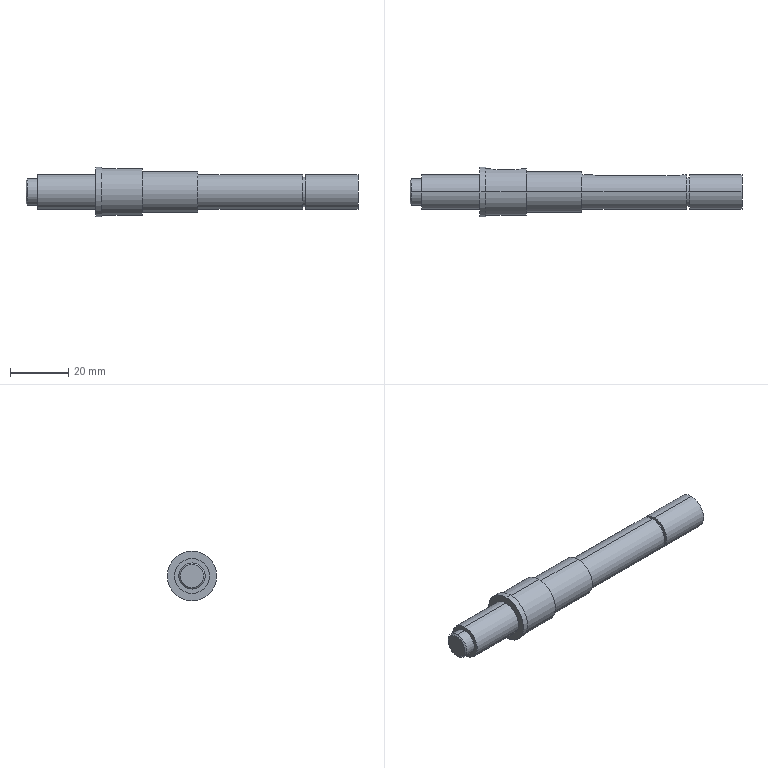Part | SolidWorks | features ICE 2, Revolution 1 | 1 solid | 39 faces | box 114 x 17 x 17 mm | volume 14497 mm3 | cylinder 22 | plane 15 | cone 2 | commonest cylinder face diameters 12 x6 4 x3 5 x3 9 x2 10 x2 14 x2
STEP:
#1=CARTESIAN_POINT('',(-42.725,5.2,0.));
#2=VERTEX_POINT('',#1);
#3=CARTESIAN_POINT('',(-40.225,5.2,2.5));
#4=VERTEX_POINT('',#3);
#5=CARTESIAN_POINT('',(-40.225,5.2,0.));
#6=DIRECTION('',(0.,1.,0.));
#7=DIRECTION('',(-1.,0.,0.));
#8=AXIS2_PLACEMENT_3D('',#5,#6,#7);
#9=CIRCLE('',#8,2.5);
#10=EDGE_CURVE('',#2,#4,#9,.T.);
#11=ORIENTED_EDGE('',*,*,#10,.F.);
#12=CARTESIAN_POINT('',(-42.725,8.,0.));
#13=VERTEX_POINT('',#12);
#14=CARTESIAN_POINT('',(-42.725,5.2,0.));
#15=DIRECTION('',(0.,1.,0.));
#16=VECTOR('',#15,1000.);
#17=LINE('',#14,#16);
#18=EDGE_CURVE('',#2,#13,#17,.T.);
#19=ORIENTED_EDGE('',*,*,#18,.T.);
#20=CARTESIAN_POINT('',(-40.225,7.599,2.5));
#21=VERTEX_POINT('',#20);
#22=CARTESIAN_POINT('',(-40.225,7.599,2.5));
#23=CARTESIAN_POINT('',(-40.392,7.599,2.5));
#24=CARTESIAN_POINT('',(-40.555,7.605,2.484));
#25=CARTESIAN_POINT('',(-40.876,7.625,2.419));
#26=CARTESIAN_POINT('',(-41.035,7.641,2.371));
#27=CARTESIAN_POINT('',(-41.338,7.679,2.245));
#28=CARTESIAN_POINT('',(-41.481,7.701,2.168));
#29=CARTESIAN_POINT('',(-41.752,7.75,1.986));
#30=CARTESIAN_POINT('',(-41.879,7.776,1.882));
#31=CARTESIAN_POINT('',(-42.223,7.854,1.538));
#32=CARTESIAN_POINT('',(-42.409,7.906,1.26));
#33=CARTESIAN_POINT('',(-42.596,7.96,0.8095));
#34=CARTESIAN_POINT('',(-42.645,7.975,0.6507));
#35=CARTESIAN_POINT('',(-42.709,7.995,0.3273));
#36=CARTESIAN_POINT('',(-42.725,8.,0.1643));
#37=CARTESIAN_POINT('',(-42.725,8.,0.));
#38=B_SPLINE_CURVE_WITH_KNOTS('',3,(#22,#23,#24,#25,#26,#27,#28,#29,#30,#31,#32,#33,#34,#35,#36,#37),.UNSPECIFIED.,.F.,.F.,(4,2,2,2,2,2,2,4),(0.,0.0004917,0.0009835,0.001475,0.001967,0.00295,0.003442,0.003934),.UNSPECIFIED.);
#39=EDGE_CURVE('',#21,#13,#38,.T.);
#40=ORIENTED_EDGE('',*,*,#39,.F.);
#41=CARTESIAN_POINT('',(-40.225,5.2,2.5));
#42=DIRECTION('',(0.,1.,0.));
#43=VECTOR('',#42,1000.);
#44=LINE('',#41,#43);
#45=EDGE_CURVE('',#4,#21,#44,.T.);
#46=ORIENTED_EDGE('',*,*,#45,.F.);
#47=EDGE_LOOP('',(#11,#19,#40,#46));
#48=FACE_OUTER_BOUND('',#47,.T.);
#49=CARTESIAN_POINT('',(-40.225,5.2,0.));
#50=DIRECTION('',(0.,1.,0.));
#51=DIRECTION('',(-1.,0.,0.));
#52=AXIS2_PLACEMENT_3D('',#49,#50,#51);
#53=CYLINDRICAL_SURFACE('',#52,2.5);
#54=ADVANCED_FACE('',(#48),#53,.F.);
#55=CARTESIAN_POINT('',(-8.054,3.8,0.));
#56=VERTEX_POINT('',#55);
#57=CARTESIAN_POINT('',(-6.054,3.8,2.));
#58=VERTEX_POINT('',#57);
#59=CARTESIAN_POINT('',(-6.054,3.8,0.));
#60=DIRECTION('',(0.,1.,0.));
#61=DIRECTION('',(-1.,0.,0.));
#62=AXIS2_PLACEMENT_3D('',#59,#60,#61);
#63=CIRCLE('',#62,2.);
#64=EDGE_CURVE('',#56,#58,#63,.T.);
#65=ORIENTED_EDGE('',*,*,#64,.F.);
#66=CARTESIAN_POINT('',(-8.054,6.,0.));
#67=VERTEX_POINT('',#66);
#68=CARTESIAN_POINT('',(-8.054,3.8,0.));
#69=DIRECTION('',(0.,1.,0.));
#70=VECTOR('',#69,1000.);
#71=LINE('',#68,#70);
#72=EDGE_CURVE('',#56,#67,#71,.T.);
#73=ORIENTED_EDGE('',*,*,#72,.T.);
#74=CARTESIAN_POINT('',(-6.054,5.657,2.));
#75=VERTEX_POINT('',#74);
#76=CARTESIAN_POINT('',(-6.054,5.657,2.));
#77=CARTESIAN_POINT('',(-6.187,5.657,2.));
#78=CARTESIAN_POINT('',(-6.318,5.662,1.987));
#79=CARTESIAN_POINT('',(-6.575,5.679,1.935));
#80=CARTESIAN_POINT('',(-6.702,5.693,1.896));
#81=CARTESIAN_POINT('',(-6.944,5.725,1.796));
#82=CARTESIAN_POINT('',(-7.059,5.744,1.734));
#83=CARTESIAN_POINT('',(-7.275,5.786,1.589));
#84=CARTESIAN_POINT('',(-7.377,5.809,1.505));
#85=CARTESIAN_POINT('',(-7.652,5.876,1.23));
#86=CARTESIAN_POINT('',(-7.8,5.92,1.009));
#87=CARTESIAN_POINT('',(-7.95,5.966,0.648));
#88=CARTESIAN_POINT('',(-7.989,5.979,0.5209));
#89=CARTESIAN_POINT('',(-8.041,5.996,0.2621));
#90=CARTESIAN_POINT('',(-8.054,6.,0.1316));
#91=CARTESIAN_POINT('',(-8.054,6.,0.));
#92=B_SPLINE_CURVE_WITH_KNOTS('',3,(#76,#77,#78,#79,#80,#81,#82,#83,#84,#85,#86,#87,#88,#89,#90,#91),.UNSPECIFIED.,.F.,.F.,(4,2,2,2,2,2,2,4),(0.,0.0003937,0.0007875,0.001181,0.001575,0.002362,0.002756,0.00315),.UNSPECIFIED.);
#93=EDGE_CURVE('',#75,#67,#92,.T.);
#94=ORIENTED_EDGE('',*,*,#93,.F.);
#95=CARTESIAN_POINT('',(-6.054,3.8,2.));
#96=DIRECTION('',(0.,1.,0.));
#97=VECTOR('',#96,1000.);
#98=LINE('',#95,#97);
#99=EDGE_CURVE('',#58,#75,#98,.T.);
#100=ORIENTED_EDGE('',*,*,#99,.F.);
#101=EDGE_LOOP('',(#65,#73,#94,#100));
#102=FACE_OUTER_BOUND('',#101,.T.);
#103=CARTESIAN_POINT('',(-6.054,3.8,0.));
#104=DIRECTION('',(0.,1.,0.));
#105=DIRECTION('',(-1.,0.,0.));
#106=AXIS2_PLACEMENT_3D('',#103,#104,#105);
#107=CYLINDRICAL_SURFACE('',#106,2.);
#108=ADVANCED_FACE('',(#102),#107,.F.);
#109=CARTESIAN_POINT('',(43.896,0.,6.));
#110=VERTEX_POINT('',#109);
#111=CARTESIAN_POINT('',(43.896,0.,-6.));
#112=VERTEX_POINT('',#111);
#113=CARTESIAN_POINT('',(43.896,0.,0.));
#114=DIRECTION('',(-1.,0.,0.));
#115=DIRECTION('',(0.,0.,1.));
#116=AXIS2_PLACEMENT_3D('',#113,#114,#115);
#117=CIRCLE('',#116,6.);
#118=EDGE_CURVE('',#110,#112,#117,.T.);
#119=ORIENTED_EDGE('',*,*,#118,.T.);
#120=CARTESIAN_POINT('',(25.896,0.,-6.));
#121=VERTEX_POINT('',#120);
#122=CARTESIAN_POINT('',(-70.104,0.,-6.));
#123=DIRECTION('',(-1.,0.,0.));
#124=VECTOR('',#123,1000.);
#125=LINE('',#122,#124);
#126=EDGE_CURVE('',#112,#121,#125,.T.);
#127=ORIENTED_EDGE('',*,*,#126,.T.);
#128=CARTESIAN_POINT('',(25.896,0.,6.));
#129=VERTEX_POINT('',#128);
#130=CARTESIAN_POINT('',(25.896,0.,0.));
#131=DIRECTION('',(-1.,0.,0.));
#132=DIRECTION('',(0.,0.,1.));
#133=AXIS2_PLACEMENT_3D('',#130,#131,#132);
#134=CIRCLE('',#133,6.);
#135=EDGE_CURVE('',#129,#121,#134,.T.);
#136=ORIENTED_EDGE('',*,*,#135,.F.);
#137=CARTESIAN_POINT('',(-70.104,0.,6.));
#138=DIRECTION('',(-1.,0.,0.));
#139=VECTOR('',#138,1000.);
#140=LINE('',#137,#139);
#141=EDGE_CURVE('',#110,#129,#140,.T.);
#142=ORIENTED_EDGE('',*,*,#141,.F.);
#143=EDGE_LOOP('',(#119,#127,#136,#142));
#144=FACE_OUTER_BOUND('',#143,.T.);
#145=CARTESIAN_POINT('',(-70.104,0.,0.));
#146=DIRECTION('',(-1.,0.,0.));
#147=DIRECTION('',(0.,0.,1.));
#148=AXIS2_PLACEMENT_3D('',#145,#146,#147);
#149=CYLINDRICAL_SURFACE('',#148,6.);
#150=ADVANCED_FACE('',(#144),#149,.T.);
#151=CARTESIAN_POINT('',(25.896,0.,5.));
#152=VERTEX_POINT('',#151);
#153=CARTESIAN_POINT('',(25.896,0.,-5.));
#154=VERTEX_POINT('',#153);
#155=CARTESIAN_POINT('',(25.896,0.,0.));
#156=DIRECTION('',(-1.,0.,0.));
#157=DIRECTION('',(0.,0.,1.));
#158=AXIS2_PLACEMENT_3D('',#155,#156,#157);
#159=CIRCLE('',#158,5.);
#160=EDGE_CURVE('',#152,#154,#159,.T.);
#161=ORIENTED_EDGE('',*,*,#160,.T.);
#162=CARTESIAN_POINT('',(24.896,0.,-5.));
#163=VERTEX_POINT('',#162);
#164=CARTESIAN_POINT('',(-70.104,0.,-5.));
#165=DIRECTION('',(-1.,0.,0.));
#166=VECTOR('',#165,1000.);
#167=LINE('',#164,#166);
#168=EDGE_CURVE('',#154,#163,#167,.T.);
#169=ORIENTED_EDGE('',*,*,#168,.T.);
#170=CARTESIAN_POINT('',(24.896,0.,5.));
#171=VERTEX_POINT('',#170);
#172=CARTESIAN_POINT('',(24.896,0.,0.));
#173=DIRECTION('',(-1.,0.,0.));
#174=DIRECTION('',(0.,0.,1.));
#175=AXIS2_PLACEMENT_3D('',#172,#173,#174);
#176=CIRCLE('',#175,5.);
#177=EDGE_CURVE('',#171,#163,#176,.T.);
#178=ORIENTED_EDGE('',*,*,#177,.F.);
#179=CARTESIAN_POINT('',(-70.104,0.,5.));
#180=DIRECTION('',(-1.,0.,0.));
#181=VECTOR('',#180,1000.);
#182=LINE('',#179,#181);
#183=EDGE_CURVE('',#152,#171,#182,.T.);
#184=ORIENTED_EDGE('',*,*,#183,.F.);
#185=EDGE_LOOP('',(#161,#169,#178,#184));
#186=FACE_OUTER_BOUND('',#185,.T.);
#187=CARTESIAN_POINT('',(-70.104,0.,0.));
#188=DIRECTION('',(-1.,0.,0.));
#189=DIRECTION('',(0.,0.,1.));
#190=AXIS2_PLACEMENT_3D('',#187,#188,#189);
#191=CYLINDRICAL_SURFACE('',#190,5.);
#192=ADVANCED_FACE('',(#186),#191,.T.);
#193=CARTESIAN_POINT('',(-6.054,5.657,-2.));
#194=VERTEX_POINT('',#193);
#195=CARTESIAN_POINT('',(21.946,5.657,-2.));
#196=VERTEX_POINT('',#195);
#197=CARTESIAN_POINT('',(-70.104,5.657,-2.));
#198=DIRECTION('',(1.,0.,0.));
#199=VECTOR('',#198,1000.);
#200=LINE('',#197,#199);
#201=EDGE_CURVE('',#194,#196,#200,.T.);
#202=ORIENTED_EDGE('',*,*,#201,.T.);
#203=CARTESIAN_POINT('',(21.946,5.657,2.));
#204=VERTEX_POINT('',#203);
#205=CARTESIAN_POINT('',(21.946,5.657,-2.));
#206=CARTESIAN_POINT('',(22.079,5.657,-2.));
#207=CARTESIAN_POINT('',(22.21,5.662,-1.987));
#208=CARTESIAN_POINT('',(22.467,5.679,-1.935));
#209=CARTESIAN_POINT('',(22.594,5.693,-1.897));
#210=CARTESIAN_POINT('',(22.836,5.725,-1.796));
#211=CARTESIAN_POINT('',(22.95,5.744,-1.735));
#212=CARTESIAN_POINT('',(23.167,5.786,-1.59));
#213=CARTESIAN_POINT('',(23.269,5.809,-1.506));
#214=CARTESIAN_POINT('',(23.543,5.875,-1.231));
#215=CARTESIAN_POINT('',(23.692,5.919,-1.01));
#216=CARTESIAN_POINT('',(23.842,5.966,-0.6496));
#217=CARTESIAN_POINT('',(23.881,5.979,-0.5226));
#218=CARTESIAN_POINT('',(23.933,5.996,-0.264));
#219=CARTESIAN_POINT('',(23.946,6.,-0.1336));
#220=CARTESIAN_POINT('',(23.946,6.,0.1294));
#221=CARTESIAN_POINT('',(23.933,5.996,0.2629));
#222=CARTESIAN_POINT('',(23.882,5.979,0.5202));
#223=CARTESIAN_POINT('',(23.844,5.966,0.6454));
#224=CARTESIAN_POINT('',(23.743,5.935,0.8889));
#225=CARTESIAN_POINT('',(23.681,5.916,1.004));
#226=CARTESIAN_POINT('',(23.536,5.876,1.22));
#227=CARTESIAN_POINT('',(23.453,5.853,1.322));
#228=CARTESIAN_POINT('',(23.269,5.809,1.506));
#229=CARTESIAN_POINT('',(23.169,5.787,1.588));
#230=CARTESIAN_POINT('',(22.953,5.745,1.733));
#231=CARTESIAN_POINT('',(22.836,5.725,1.796));
#232=CARTESIAN_POINT('',(22.475,5.677,1.946));
#233=CARTESIAN_POINT('',(22.212,5.657,2.));
#234=CARTESIAN_POINT('',(21.946,5.657,2.));
#235=B_SPLINE_CURVE_WITH_KNOTS('',3,(#205,#206,#207,#208,#209,#210,#211,#212,#213,#214,#215,#216,#217,#218,#219,#220,#221,#222,#223,#224,#225,#226,#227,#228,#229,#230,#231,#232,#233,#234),.UNSPECIFIED.,.F.,.F.,(4,2,2,2,2,2,2,2,2,2,2,2,2,2,4),(0.,0.0003935,0.000787,0.00118,0.001574,0.002361,0.002754,0.003148,0.003541,0.003935,0.004328,0.004722,0.005115,0.005509,0.006296),.UNSPECIFIED.);
#236=EDGE_CURVE('',#196,#204,#235,.T.);
#237=ORIENTED_EDGE('',*,*,#236,.T.);
#238=CARTESIAN_POINT('',(-70.104,5.657,2.));
#239=DIRECTION('',(-1.,0.,0.));
#240=VECTOR('',#239,1000.);
#241=LINE('',#238,#240);
#242=EDGE_CURVE('',#204,#75,#241,.T.);
#243=ORIENTED_EDGE('',*,*,#242,.T.);
#244=ORIENTED_EDGE('',*,*,#93,.T.);
#245=CARTESIAN_POINT('',(-8.054,6.,0.));
#246=CARTESIAN_POINT('',(-8.054,6.,-0.1314));
#247=CARTESIAN_POINT('',(-8.041,5.996,-0.2649));
#248=CARTESIAN_POINT('',(-7.989,5.979,-0.5219));
#249=CARTESIAN_POINT('',(-7.951,5.966,-0.647));
#250=CARTESIAN_POINT('',(-7.85,5.935,-0.8902));
#251=CARTESIAN_POINT('',(-7.788,5.916,-1.006));
#252=CARTESIAN_POINT('',(-7.643,5.875,-1.221));
#253=CARTESIAN_POINT('',(-7.56,5.853,-1.323));
#254=CARTESIAN_POINT('',(-7.376,5.809,-1.507));
#255=CARTESIAN_POINT('',(-7.276,5.786,-1.589));
#256=CARTESIAN_POINT('',(-7.06,5.745,-1.733));
#257=CARTESIAN_POINT('',(-6.943,5.725,-1.796));
#258=CARTESIAN_POINT('',(-6.583,5.677,-1.946));
#259=CARTESIAN_POINT('',(-6.32,5.657,-2.));
#260=CARTESIAN_POINT('',(-6.054,5.657,-2.));
#261=B_SPLINE_CURVE_WITH_KNOTS('',3,(#245,#246,#247,#248,#249,#250,#251,#252,#253,#254,#255,#256,#257,#258,#259,#260),.UNSPECIFIED.,.F.,.F.,(4,2,2,2,2,2,2,4),(0.00315,0.003543,0.003936,0.00433,0.004723,0.005116,0.005509,0.006296),.UNSPECIFIED.);
#262=EDGE_CURVE('',#67,#194,#261,.T.);
#263=ORIENTED_EDGE('',*,*,#262,.T.);
#264=EDGE_LOOP('',(#202,#237,#243,#244,#263));
#265=FACE_BOUND('',#264,.T.);
#266=CARTESIAN_POINT('',(24.896,0.,6.));
#267=VERTEX_POINT('',#266);
#268=CARTESIAN_POINT('',(24.896,0.,-6.));
#269=VERTEX_POINT('',#268);
#270=CARTESIAN_POINT('',(24.896,0.,0.));
#271=DIRECTION('',(-1.,0.,0.));
#272=DIRECTION('',(0.,0.,1.));
#273=AXIS2_PLACEMENT_3D('',#270,#271,#272);
#274=CIRCLE('',#273,6.);
#275=EDGE_CURVE('',#267,#269,#274,.T.);
#276=ORIENTED_EDGE('',*,*,#275,.T.);
#277=CARTESIAN_POINT('',(-11.104,0.,-6.));
#278=VERTEX_POINT('',#277);
#279=CARTESIAN_POINT('',(-70.104,0.,-6.));
#280=DIRECTION('',(-1.,0.,0.));
#281=VECTOR('',#280,1000.);
#282=LINE('',#279,#281);
#283=EDGE_CURVE('',#269,#278,#282,.T.);
#284=ORIENTED_EDGE('',*,*,#283,.T.);
#285=CARTESIAN_POINT('',(-11.104,0.,6.));
#286=VERTEX_POINT('',#285);
#287=CARTESIAN_POINT('',(-11.104,0.,0.));
#288=DIRECTION('',(-1.,0.,0.));
#289=DIRECTION('',(0.,0.,1.));
#290=AXIS2_PLACEMENT_3D('',#287,#288,#289);
#291=CIRCLE('',#290,6.);
#292=EDGE_CURVE('',#286,#278,#291,.T.);
#293=ORIENTED_EDGE('',*,*,#292,.F.);
#294=CARTESIAN_POINT('',(-70.104,0.,6.));
#295=DIRECTION('',(-1.,0.,0.));
#296=VECTOR('',#295,1000.);
#297=LINE('',#294,#296);
#298=EDGE_CURVE('',#267,#286,#297,.T.);
#299=ORIENTED_EDGE('',*,*,#298,.F.);
#300=EDGE_LOOP('',(#276,#284,#293,#299));
#301=FACE_OUTER_BOUND('',#300,.T.);
#302=CARTESIAN_POINT('',(-70.104,0.,0.));
#303=DIRECTION('',(-1.,0.,0.));
#304=DIRECTION('',(0.,0.,1.));
#305=AXIS2_PLACEMENT_3D('',#302,#303,#304);
#306=CYLINDRICAL_SURFACE('',#305,6.);
#307=ADVANCED_FACE('',(#265,#301),#306,.T.);
#308=CARTESIAN_POINT('',(-11.104,0.,7.));
#309=VERTEX_POINT('',#308);
#310=CARTESIAN_POINT('',(-11.104,0.,-7.));
#311=VERTEX_POINT('',#310);
#312=CARTESIAN_POINT('',(-11.104,0.,0.));
#313=DIRECTION('',(-1.,0.,0.));
#314=DIRECTION('',(0.,0.,1.));
#315=AXIS2_PLACEMENT_3D('',#312,#313,#314);
#316=CIRCLE('',#315,7.);
#317=EDGE_CURVE('',#309,#311,#316,.T.);
#318=ORIENTED_EDGE('',*,*,#317,.T.);
#319=CARTESIAN_POINT('',(-30.104,0.,-7.));
#320=VERTEX_POINT('',#319);
#321=CARTESIAN_POINT('',(-70.104,0.,-7.));
#322=DIRECTION('',(-1.,0.,0.));
#323=VECTOR('',#322,1000.);
#324=LINE('',#321,#323);
#325=EDGE_CURVE('',#311,#320,#324,.T.);
#326=ORIENTED_EDGE('',*,*,#325,.T.);
#327=CARTESIAN_POINT('',(-30.104,0.,7.));
#328=VERTEX_POINT('',#327);
#329=CARTESIAN_POINT('',(-30.104,0.,0.));
#330=DIRECTION('',(-1.,0.,0.));
#331=DIRECTION('',(0.,0.,1.));
#332=AXIS2_PLACEMENT_3D('',#329,#330,#331);
#333=CIRCLE('',#332,7.);
#334=EDGE_CURVE('',#328,#320,#333,.T.);
#335=ORIENTED_EDGE('',*,*,#334,.F.);
#336=CARTESIAN_POINT('',(-70.104,0.,7.));
#337=DIRECTION('',(-1.,0.,0.));
#338=VECTOR('',#337,1000.);
#339=LINE('',#336,#338);
#340=EDGE_CURVE('',#309,#328,#339,.T.);
#341=ORIENTED_EDGE('',*,*,#340,.F.);
#342=EDGE_LOOP('',(#318,#326,#335,#341));
#343=FACE_OUTER_BOUND('',#342,.T.);
#344=CARTESIAN_POINT('',(-70.104,0.,0.));
#345=DIRECTION('',(-1.,0.,0.));
#346=DIRECTION('',(0.,0.,1.));
#347=AXIS2_PLACEMENT_3D('',#344,#345,#346);
#348=CYLINDRICAL_SURFACE('',#347,7.);
#349=ADVANCED_FACE('',(#343),#348,.T.);
#350=CARTESIAN_POINT('',(-40.225,7.599,-2.5));
#351=VERTEX_POINT('',#350);
#352=CARTESIAN_POINT('',(-34.104,7.599,-2.5));
#353=VERTEX_POINT('',#352);
#354=CARTESIAN_POINT('',(-70.104,7.599,-2.5));
#355=DIRECTION('',(1.,0.,0.));
#356=VECTOR('',#355,1000.);
#357=LINE('',#354,#356);
#358=EDGE_CURVE('',#351,#353,#357,.T.);
#359=ORIENTED_EDGE('',*,*,#358,.T.);
#360=CARTESIAN_POINT('',(-34.104,7.599,2.5));
#361=VERTEX_POINT('',#360);
#362=CARTESIAN_POINT('',(-34.104,7.599,-2.5));
#363=CARTESIAN_POINT('',(-33.938,7.599,-2.5));
#364=CARTESIAN_POINT('',(-33.774,7.605,-2.484));
#365=CARTESIAN_POINT('',(-33.454,7.625,-2.419));
#366=CARTESIAN_POINT('',(-33.294,7.641,-2.371));
#367=CARTESIAN_POINT('',(-32.992,7.679,-2.245));
#368=CARTESIAN_POINT('',(-32.849,7.701,-2.168));
#369=CARTESIAN_POINT('',(-32.578,7.75,-1.987));
#370=CARTESIAN_POINT('',(-32.451,7.776,-1.882));
#371=CARTESIAN_POINT('',(-32.107,7.854,-1.539));
#372=CARTESIAN_POINT('',(-31.921,7.906,-1.262));
#373=CARTESIAN_POINT('',(-31.734,7.96,-0.8114));
#374=CARTESIAN_POINT('',(-31.685,7.975,-0.6527));
#375=CARTESIAN_POINT('',(-31.62,7.995,-0.3296));
#376=CARTESIAN_POINT('',(-31.604,8.,-0.1667));
#377=CARTESIAN_POINT('',(-31.604,8.,0.1617));
#378=CARTESIAN_POINT('',(-31.62,7.995,0.3285));
#379=CARTESIAN_POINT('',(-31.684,7.975,0.6499));
#380=CARTESIAN_POINT('',(-31.732,7.961,0.8063));
#381=CARTESIAN_POINT('',(-31.858,7.924,1.11));
#382=CARTESIAN_POINT('',(-31.936,7.902,1.255));
#383=CARTESIAN_POINT('',(-32.116,7.855,1.525));
#384=CARTESIAN_POINT('',(-32.22,7.828,1.652));
#385=CARTESIAN_POINT('',(-32.451,7.776,1.883));
#386=CARTESIAN_POINT('',(-32.576,7.75,1.985));
#387=CARTESIAN_POINT('',(-32.846,7.702,2.166));
#388=CARTESIAN_POINT('',(-32.992,7.679,2.245));
#389=CARTESIAN_POINT('',(-33.293,7.641,2.37));
#390=CARTESIAN_POINT('',(-33.449,7.626,2.418));
#391=CARTESIAN_POINT('',(-33.771,7.605,2.483));
#392=CARTESIAN_POINT('',(-33.938,7.599,2.5));
#393=CARTESIAN_POINT('',(-34.104,7.599,2.5));
#394=B_SPLINE_CURVE_WITH_KNOTS('',3,(#362,#363,#364,#365,#366,#367,#368,#369,#370,#371,#372,#373,#374,#375,#376,#377,#378,#379,#380,#381,#382,#383,#384,#385,#386,#387,#388,#389,#390,#391,#392,#393),.UNSPECIFIED.,.F.,.F.,(4,2,2,2,2,2,2,2,2,2,2,2,2,2,2,4),(0.,0.0004914,0.0009828,0.001474,0.001966,0.002949,0.00344,0.003931,0.004423,0.004914,0.005406,0.005897,0.006388,0.00688,0.007371,0.007863),.UNSPECIFIED.);
#395=EDGE_CURVE('',#353,#361,#394,.T.);
#396=ORIENTED_EDGE('',*,*,#395,.T.);
#397=CARTESIAN_POINT('',(-70.104,7.599,2.5));
#398=DIRECTION('',(-1.,0.,0.));
#399=VECTOR('',#398,1000.);
#400=LINE('',#397,#399);
#401=EDGE_CURVE('',#361,#21,#400,.T.);
#402=ORIENTED_EDGE('',*,*,#401,.T.);
#403=ORIENTED_EDGE('',*,*,#39,.T.);
#404=CARTESIAN_POINT('',(-42.725,8.,0.));
#405=CARTESIAN_POINT('',(-42.725,8.,-0.1641));
#406=CARTESIAN_POINT('',(-42.709,7.995,-0.3308));
#407=CARTESIAN_POINT('',(-42.644,7.975,-0.652));
#408=CARTESIAN_POINT('',(-42.597,7.961,-0.8082));
#409=CARTESIAN_POINT('',(-42.47,7.924,-1.112));
#410=CARTESIAN_POINT('',(-42.393,7.902,-1.256));
#411=CARTESIAN_POINT('',(-42.212,7.854,-1.526));
#412=CARTESIAN_POINT('',(-42.108,7.828,-1.653));
#413=CARTESIAN_POINT('',(-41.878,7.776,-1.883));
#414=CARTESIAN_POINT('',(-41.753,7.75,-1.986));
#415=CARTESIAN_POINT('',(-41.483,7.702,-2.167));
#416=CARTESIAN_POINT('',(-41.337,7.679,-2.245));
#417=CARTESIAN_POINT('',(-41.036,7.641,-2.371));
#418=CARTESIAN_POINT('',(-40.88,7.626,-2.418));
#419=CARTESIAN_POINT('',(-40.558,7.605,-2.483));
#420=CARTESIAN_POINT('',(-40.392,7.599,-2.5));
#421=CARTESIAN_POINT('',(-40.225,7.599,-2.5));
#422=B_SPLINE_CURVE_WITH_KNOTS('',3,(#404,#405,#406,#407,#408,#409,#410,#411,#412,#413,#414,#415,#416,#417,#418,#419,#420,#421),.UNSPECIFIED.,.F.,.F.,(4,2,2,2,2,2,2,2,4),(0.003934,0.004425,0.004916,0.005407,0.005898,0.006389,0.006881,0.007372,0.007863),.UNSPECIFIED.);
#423=EDGE_CURVE('',#13,#351,#422,.T.);
#424=ORIENTED_EDGE('',*,*,#423,.T.);
#425=EDGE_LOOP('',(#359,#396,#402,#403,#424));
#426=FACE_BOUND('',#425,.T.);
#427=CARTESIAN_POINT('',(-30.104,0.,8.));
#428=VERTEX_POINT('',#427);
#429=CARTESIAN_POINT('',(-30.104,0.,-8.));
#430=VERTEX_POINT('',#429);
#431=CARTESIAN_POINT('',(-30.104,0.,0.));
#432=DIRECTION('',(-1.,0.,0.));
#433=DIRECTION('',(0.,0.,1.));
#434=AXIS2_PLACEMENT_3D('',#431,#432,#433);
#435=CIRCLE('',#434,8.);
#436=EDGE_CURVE('',#428,#430,#435,.T.);
#437=ORIENTED_EDGE('',*,*,#436,.T.);
#438=CARTESIAN_POINT('',(-44.104,0.,-8.));
#439=VERTEX_POINT('',#438);
#440=CARTESIAN_POINT('',(-70.104,0.,-8.));
#441=DIRECTION('',(-1.,0.,0.));
#442=VECTOR('',#441,1000.);
#443=LINE('',#440,#442);
#444=EDGE_CURVE('',#430,#439,#443,.T.);
#445=ORIENTED_EDGE('',*,*,#444,.T.);
#446=CARTESIAN_POINT('',(-44.104,0.,8.));
#447=VERTEX_POINT('',#446);
#448=CARTESIAN_POINT('',(-44.104,0.,0.));
#449=DIRECTION('',(-1.,0.,0.));
#450=DIRECTION('',(0.,0.,1.));
#451=AXIS2_PLACEMENT_3D('',#448,#449,#450);
#452=CIRCLE('',#451,8.);
#453=EDGE_CURVE('',#447,#439,#452,.T.);
#454=ORIENTED_EDGE('',*,*,#453,.F.);
#455=CARTESIAN_POINT('',(-70.104,0.,8.));
#456=DIRECTION('',(-1.,0.,0.));
#457=VECTOR('',#456,1000.);
#458=LINE('',#455,#457);
#459=EDGE_CURVE('',#428,#447,#458,.T.);
#460=ORIENTED_EDGE('',*,*,#459,.F.);
#461=EDGE_LOOP('',(#437,#445,#454,#460));
#462=FACE_OUTER_BOUND('',#461,.T.);
#463=CARTESIAN_POINT('',(-70.104,0.,0.));
#464=DIRECTION('',(-1.,0.,0.));
#465=DIRECTION('',(0.,0.,1.));
#466=AXIS2_PLACEMENT_3D('',#463,#464,#465);
#467=CYLINDRICAL_SURFACE('',#466,8.);
#468=ADVANCED_FACE('',(#426,#462),#467,.T.);
#469=CARTESIAN_POINT('',(-44.104,0.,8.5));
#470=VERTEX_POINT('',#469);
#471=CARTESIAN_POINT('',(-44.104,0.,-8.5));
#472=VERTEX_POINT('',#471);
#473=CARTESIAN_POINT('',(-44.104,0.,0.));
#474=DIRECTION('',(-1.,0.,0.));
#475=DIRECTION('',(0.,0.,1.));
#476=AXIS2_PLACEMENT_3D('',#473,#474,#475);
#477=CIRCLE('',#476,8.5);
#478=EDGE_CURVE('',#470,#472,#477,.T.);
#479=ORIENTED_EDGE('',*,*,#478,.T.);
#480=CARTESIAN_POINT('',(-46.104,0.,-8.5));
#481=VERTEX_POINT('',#480);
#482=CARTESIAN_POINT('',(-70.104,0.,-8.5));
#483=DIRECTION('',(-1.,0.,0.));
#484=VECTOR('',#483,1000.);
#485=LINE('',#482,#484);
#486=EDGE_CURVE('',#472,#481,#485,.T.);
#487=ORIENTED_EDGE('',*,*,#486,.T.);
#488=CARTESIAN_POINT('',(-46.104,0.,8.5));
#489=VERTEX_POINT('',#488);
#490=CARTESIAN_POINT('',(-46.104,0.,0.));
#491=DIRECTION('',(-1.,0.,0.));
#492=DIRECTION('',(0.,0.,1.));
#493=AXIS2_PLACEMENT_3D('',#490,#491,#492);
#494=CIRCLE('',#493,8.5);
#495=EDGE_CURVE('',#489,#481,#494,.T.);
#496=ORIENTED_EDGE('',*,*,#495,.F.);
#497=CARTESIAN_POINT('',(-70.104,0.,8.5));
#498=DIRECTION('',(-1.,0.,0.));
#499=VECTOR('',#498,1000.);
#500=LINE('',#497,#499);
#501=EDGE_CURVE('',#470,#489,#500,.T.);
#502=ORIENTED_EDGE('',*,*,#501,.F.);
#503=EDGE_LOOP('',(#479,#487,#496,#502));
#504=FACE_OUTER_BOUND('',#503,.T.);
#505=CARTESIAN_POINT('',(-70.104,0.,0.));
#506=DIRECTION('',(-1.,0.,0.));
#507=DIRECTION('',(0.,0.,1.));
#508=AXIS2_PLACEMENT_3D('',#505,#506,#507);
#509=CYLINDRICAL_SURFACE('',#508,8.5);
#510=ADVANCED_FACE('',(#504),#509,.T.);
#511=CARTESIAN_POINT('',(-46.104,0.,6.));
#512=VERTEX_POINT('',#511);
#513=CARTESIAN_POINT('',(-46.104,0.,-6.));
#514=VERTEX_POINT('',#513);
#515=CARTESIAN_POINT('',(-46.104,0.,0.));
#516=DIRECTION('',(-1.,0.,0.));
#517=DIRECTION('',(0.,0.,1.));
#518=AXIS2_PLACEMENT_3D('',#515,#516,#517);
#519=CIRCLE('',#518,6.);
#520=EDGE_CURVE('',#512,#514,#519,.T.);
#521=ORIENTED_EDGE('',*,*,#520,.T.);
#522=CARTESIAN_POINT('',(-66.104,0.,-6.));
#523=VERTEX_POINT('',#522);
#524=CARTESIAN_POINT('',(-70.104,0.,-6.));
#525=DIRECTION('',(-1.,0.,0.));
#526=VECTOR('',#525,1000.);
#527=LINE('',#524,#526);
#528=EDGE_CURVE('',#514,#523,#527,.T.);
#529=ORIENTED_EDGE('',*,*,#528,.T.);
#530=CARTESIAN_POINT('',(-66.104,0.,6.));
#531=VERTEX_POINT('',#530);
#532=CARTESIAN_POINT('',(-66.104,0.,0.));
#533=DIRECTION('',(-1.,0.,0.));
#534=DIRECTION('',(0.,0.,1.));
#535=AXIS2_PLACEMENT_3D('',#532,#533,#534);
#536=CIRCLE('',#535,6.);
#537=EDGE_CURVE('',#531,#523,#536,.T.);
#538=ORIENTED_EDGE('',*,*,#537,.F.);
#539=CARTESIAN_POINT('',(-70.104,0.,6.));
#540=DIRECTION('',(-1.,0.,0.));
#541=VECTOR('',#540,1000.);
#542=LINE('',#539,#541);
#543=EDGE_CURVE('',#512,#531,#542,.T.);
#544=ORIENTED_EDGE('',*,*,#543,.F.);
#545=EDGE_LOOP('',(#521,#529,#538,#544));
#546=FACE_OUTER_BOUND('',#545,.T.);
#547=CARTESIAN_POINT('',(-70.104,0.,0.));
#548=DIRECTION('',(-1.,0.,0.));
#549=DIRECTION('',(0.,0.,1.));
#550=AXIS2_PLACEMENT_3D('',#547,#548,#549);
#551=CYLINDRICAL_SURFACE('',#550,6.);
#552=ADVANCED_FACE('',(#546),#551,.T.);
#553=CARTESIAN_POINT('',(-66.104,0.,4.5));
#554=VERTEX_POINT('',#553);
#555=CARTESIAN_POINT('',(-66.104,0.,-4.5));
#556=VERTEX_POINT('',#555);
#557=CARTESIAN_POINT('',(-66.104,0.,0.));
#558=DIRECTION('',(-1.,0.,0.));
#559=DIRECTION('',(0.,0.,1.));
#560=AXIS2_PLACEMENT_3D('',#557,#558,#559);
#561=CIRCLE('',#560,4.5);
#562=EDGE_CURVE('',#554,#556,#561,.T.);
#563=ORIENTED_EDGE('',*,*,#562,.T.);
#564=CARTESIAN_POINT('',(-69.604,0.,-4.5));
#565=VERTEX_POINT('',#564);
#566=CARTESIAN_POINT('',(-70.104,0.,-4.5));
#567=DIRECTION('',(-1.,0.,0.));
#568=VECTOR('',#567,1000.);
#569=LINE('',#566,#568);
#570=EDGE_CURVE('',#556,#565,#569,.T.);
#571=ORIENTED_EDGE('',*,*,#570,.T.);
#572=CARTESIAN_POINT('',(-69.604,0.,4.5));
#573=VERTEX_POINT('',#572);
#574=CARTESIAN_POINT('',(-69.604,0.,0.));
#575=DIRECTION('',(-1.,0.,0.));
#576=DIRECTION('',(0.,0.,1.));
#577=AXIS2_PLACEMENT_3D('',#574,#575,#576);
#578=CIRCLE('',#577,4.5);
#579=EDGE_CURVE('',#573,#565,#578,.T.);
#580=ORIENTED_EDGE('',*,*,#579,.F.);
#581=CARTESIAN_POINT('',(-70.104,0.,4.5));
#582=DIRECTION('',(-1.,0.,0.));
#583=VECTOR('',#582,1000.);
#584=LINE('',#581,#583);
#585=EDGE_CURVE('',#554,#573,#584,.T.);
#586=ORIENTED_EDGE('',*,*,#585,.F.);
#587=EDGE_LOOP('',(#563,#571,#580,#586));
#588=FACE_OUTER_BOUND('',#587,.T.);
#589=CARTESIAN_POINT('',(-70.104,0.,0.));
#590=DIRECTION('',(-1.,0.,0.));
#591=DIRECTION('',(0.,0.,1.));
#592=AXIS2_PLACEMENT_3D('',#589,#590,#591);
#593=CYLINDRICAL_SURFACE('',#592,4.5);
#594=ADVANCED_FACE('',(#588),#593,.T.);
#595=CARTESIAN_POINT('',(-70.104,0.,4.));
#596=VERTEX_POINT('',#595);
#597=CARTESIAN_POINT('',(-70.104,0.,-4.));
#598=VERTEX_POINT('',#597);
#599=CARTESIAN_POINT('',(-70.104,0.,0.));
#600=DIRECTION('',(-1.,0.,0.));
#601=DIRECTION('',(0.,0.,1.));
#602=AXIS2_PLACEMENT_3D('',#599,#600,#601);
#603=CIRCLE('',#602,4.);
#604=EDGE_CURVE('',#596,#598,#603,.T.);
#605=ORIENTED_EDGE('',*,*,#604,.F.);
#606=CARTESIAN_POINT('',(-69.604,0.,4.5));
#607=DIRECTION('',(0.7071,0.,0.7071));
#608=VECTOR('',#607,1000.);
#609=LINE('',#606,#608);
#610=EDGE_CURVE('',#596,#573,#609,.T.);
#611=ORIENTED_EDGE('',*,*,#610,.T.);
#612=ORIENTED_EDGE('',*,*,#579,.T.);
#613=CARTESIAN_POINT('',(-69.604,0.,-4.5));
#614=DIRECTION('',(0.7071,0.,-0.7071));
#615=VECTOR('',#614,1000.);
#616=LINE('',#613,#615);
#617=EDGE_CURVE('',#598,#565,#616,.T.);
#618=ORIENTED_EDGE('',*,*,#617,.F.);
#619=EDGE_LOOP('',(#605,#611,#612,#618));
#620=FACE_OUTER_BOUND('',#619,.T.);
#621=CARTESIAN_POINT('',(-69.604,0.,0.));
#622=DIRECTION('',(1.,0.,0.));
#623=DIRECTION('',(0.,0.,-1.));
#624=AXIS2_PLACEMENT_3D('',#621,#622,#623);
#625=CONICAL_SURFACE('',#624,4.5,0.7854);
#626=ADVANCED_FACE('',(#620),#625,.T.);
#627=CARTESIAN_POINT('',(-70.104,0.,0.));
#628=DIRECTION('',(-1.,0.,0.));
#629=DIRECTION('',(0.,0.,1.));
#630=AXIS2_PLACEMENT_3D('',#627,#628,#629);
#631=CIRCLE('',#630,4.);
#632=EDGE_CURVE('',#598,#596,#631,.T.);
#633=ORIENTED_EDGE('',*,*,#632,.T.);
#634=ORIENTED_EDGE('',*,*,#604,.T.);
#635=EDGE_LOOP('',(#633,#634));
#636=FACE_OUTER_BOUND('',#635,.T.);
#637=CARTESIAN_POINT('',(-70.104,4.,0.));
#638=DIRECTION('',(1.,0.,0.));
#639=DIRECTION('',(0.,0.,-1.));
#640=AXIS2_PLACEMENT_3D('',#637,#638,#639);
#641=PLANE('',#640);
#642=ADVANCED_FACE('',(#636),#641,.F.);
#643=ORIENTED_EDGE('',*,*,#610,.F.);
#644=ORIENTED_EDGE('',*,*,#632,.F.);
#645=ORIENTED_EDGE('',*,*,#617,.T.);
#646=CARTESIAN_POINT('',(-69.604,0.,0.));
#647=DIRECTION('',(-1.,0.,0.));
#648=DIRECTION('',(0.,0.,1.));
#649=AXIS2_PLACEMENT_3D('',#646,#647,#648);
#650=CIRCLE('',#649,4.5);
#651=EDGE_CURVE('',#565,#573,#650,.T.);
#652=ORIENTED_EDGE('',*,*,#651,.T.);
#653=EDGE_LOOP('',(#643,#644,#645,#652));
#654=FACE_OUTER_BOUND('',#653,.T.);
#655=CARTESIAN_POINT('',(-69.604,0.,0.));
#656=DIRECTION('',(1.,0.,0.));
#657=DIRECTION('',(0.,0.,-1.));
#658=AXIS2_PLACEMENT_3D('',#655,#656,#657);
#659=CONICAL_SURFACE('',#658,4.5,0.7854);
#660=ADVANCED_FACE('',(#654),#659,.T.);
#661=ORIENTED_EDGE('',*,*,#570,.F.);
#662=CARTESIAN_POINT('',(-66.104,0.,0.));
#663=DIRECTION('',(-1.,0.,0.));
#664=DIRECTION('',(0.,0.,1.));
#665=AXIS2_PLACEMENT_3D('',#662,#663,#664);
#666=CIRCLE('',#665,4.5);
#667=EDGE_CURVE('',#556,#554,#666,.T.);
#668=ORIENTED_EDGE('',*,*,#667,.T.);
#669=ORIENTED_EDGE('',*,*,#585,.T.);
#670=ORIENTED_EDGE('',*,*,#651,.F.);
#671=EDGE_LOOP('',(#661,#668,#669,#670));
#672=FACE_OUTER_BOUND('',#671,.T.);
#673=CARTESIAN_POINT('',(-70.104,0.,0.));
#674=DIRECTION('',(-1.,0.,0.));
#675=DIRECTION('',(0.,0.,1.));
#676=AXIS2_PLACEMENT_3D('',#673,#674,#675);
#677=CYLINDRICAL_SURFACE('',#676,4.5);
#678=ADVANCED_FACE('',(#672),#677,.T.);
#679=ORIENTED_EDGE('',*,*,#562,.F.);
#680=ORIENTED_EDGE('',*,*,#667,.F.);
#681=EDGE_LOOP('',(#679,#680));
#682=FACE_BOUND('',#681,.T.);
#683=ORIENTED_EDGE('',*,*,#537,.T.);
#684=CARTESIAN_POINT('',(-66.104,0.,0.));
#685=DIRECTION('',(-1.,0.,0.));
#686=DIRECTION('',(0.,0.,1.));
#687=AXIS2_PLACEMENT_3D('',#684,#685,#686);
#688=CIRCLE('',#687,6.);
#689=EDGE_CURVE('',#523,#531,#688,.T.);
#690=ORIENTED_EDGE('',*,*,#689,.T.);
#691=EDGE_LOOP('',(#683,#690));
#692=FACE_OUTER_BOUND('',#691,.T.);
#693=CARTESIAN_POINT('',(-66.104,4.5,0.));
#694=DIRECTION('',(1.,0.,0.));
#695=DIRECTION('',(0.,0.,-1.));
#696=AXIS2_PLACEMENT_3D('',#693,#694,#695);
#697=PLANE('',#696);
#698=ADVANCED_FACE('',(#682,#692),#697,.F.);
#699=ORIENTED_EDGE('',*,*,#528,.F.);
#700=CARTESIAN_POINT('',(-46.104,0.,0.));
#701=DIRECTION('',(-1.,0.,0.));
#702=DIRECTION('',(0.,0.,1.));
#703=AXIS2_PLACEMENT_3D('',#700,#701,#702);
#704=CIRCLE('',#703,6.);
#705=EDGE_CURVE('',#514,#512,#704,.T.);
#706=ORIENTED_EDGE('',*,*,#705,.T.);
#707=ORIENTED_EDGE('',*,*,#543,.T.);
#708=ORIENTED_EDGE('',*,*,#689,.F.);
#709=EDGE_LOOP('',(#699,#706,#707,#708));
#710=FACE_OUTER_BOUND('',#709,.T.);
#711=CARTESIAN_POINT('',(-70.104,0.,0.));
#712=DIRECTION('',(-1.,0.,0.));
#713=DIRECTION('',(0.,0.,1.));
#714=AXIS2_PLACEMENT_3D('',#711,#712,#713);
#715=CYLINDRICAL_SURFACE('',#714,6.);
#716=ADVANCED_FACE('',(#710),#715,.T.);
#717=ORIENTED_EDGE('',*,*,#520,.F.);
#718=ORIENTED_EDGE('',*,*,#705,.F.);
#719=EDGE_LOOP('',(#717,#718));
#720=FACE_BOUND('',#719,.T.);
#721=ORIENTED_EDGE('',*,*,#495,.T.);
#722=CARTESIAN_POINT('',(-46.104,0.,0.));
#723=DIRECTION('',(-1.,0.,0.));
#724=DIRECTION('',(0.,0.,1.));
#725=AXIS2_PLACEMENT_3D('',#722,#723,#724);
#726=CIRCLE('',#725,8.5);
#727=EDGE_CURVE('',#481,#489,#726,.T.);
#728=ORIENTED_EDGE('',*,*,#727,.T.);
#729=EDGE_LOOP('',(#721,#728));
#730=FACE_OUTER_BOUND('',#729,.T.);
#731=CARTESIAN_POINT('',(-46.104,6.,0.));
#732=DIRECTION('',(1.,0.,0.));
#733=DIRECTION('',(0.,0.,-1.));
#734=AXIS2_PLACEMENT_3D('',#731,#732,#733);
#735=PLANE('',#734);
#736=ADVANCED_FACE('',(#720,#730),#735,.F.);
#737=ORIENTED_EDGE('',*,*,#486,.F.);
#738=CARTESIAN_POINT('',(-44.104,0.,0.));
#739=DIRECTION('',(-1.,0.,0.));
#740=DIRECTION('',(0.,0.,1.));
#741=AXIS2_PLACEMENT_3D('',#738,#739,#740);
#742=CIRCLE('',#741,8.5);
#743=EDGE_CURVE('',#472,#470,#742,.T.);
#744=ORIENTED_EDGE('',*,*,#743,.T.);
#745=ORIENTED_EDGE('',*,*,#501,.T.);
#746=ORIENTED_EDGE('',*,*,#727,.F.);
#747=EDGE_LOOP('',(#737,#744,#745,#746));
#748=FACE_OUTER_BOUND('',#747,.T.);
#749=CARTESIAN_POINT('',(-70.104,0.,0.));
#750=DIRECTION('',(-1.,0.,0.));
#751=DIRECTION('',(0.,0.,1.));
#752=AXIS2_PLACEMENT_3D('',#749,#750,#751);
#753=CYLINDRICAL_SURFACE('',#752,8.5);
#754=ADVANCED_FACE('',(#748),#753,.T.);
#755=ORIENTED_EDGE('',*,*,#478,.F.);
#756=ORIENTED_EDGE('',*,*,#743,.F.);
#757=EDGE_LOOP('',(#755,#756));
#758=FACE_OUTER_BOUND('',#757,.T.);
#759=ORIENTED_EDGE('',*,*,#453,.T.);
#760=CARTESIAN_POINT('',(-44.104,0.,0.));
#761=DIRECTION('',(-1.,0.,0.));
#762=DIRECTION('',(0.,0.,1.));
#763=AXIS2_PLACEMENT_3D('',#760,#761,#762);
#764=CIRCLE('',#763,8.);
#765=EDGE_CURVE('',#439,#447,#764,.T.);
#766=ORIENTED_EDGE('',*,*,#765,.T.);
#767=EDGE_LOOP('',(#759,#766));
#768=FACE_BOUND('',#767,.T.);
#769=CARTESIAN_POINT('',(-44.104,8.5,0.));
#770=DIRECTION('',(-1.,0.,0.));
#771=DIRECTION('',(0.,0.,1.));
#772=AXIS2_PLACEMENT_3D('',#769,#770,#771);
#773=PLANE('',#772);
#774=ADVANCED_FACE('',(#758,#768),#773,.F.);
#775=ORIENTED_EDGE('',*,*,#444,.F.);
#776=CARTESIAN_POINT('',(-30.104,0.,0.));
#777=DIRECTION('',(-1.,0.,0.));
#778=DIRECTION('',(0.,0.,1.));
#779=AXIS2_PLACEMENT_3D('',#776,#777,#778);
#780=CIRCLE('',#779,8.);
#781=EDGE_CURVE('',#430,#428,#780,.T.);
#782=ORIENTED_EDGE('',*,*,#781,.T.);
#783=ORIENTED_EDGE('',*,*,#459,.T.);
#784=ORIENTED_EDGE('',*,*,#765,.F.);
#785=EDGE_LOOP('',(#775,#782,#783,#784));
#786=FACE_OUTER_BOUND('',#785,.T.);
#787=CARTESIAN_POINT('',(-70.104,0.,0.));
#788=DIRECTION('',(-1.,0.,0.));
#789=DIRECTION('',(0.,0.,1.));
#790=AXIS2_PLACEMENT_3D('',#787,#788,#789);
#791=CYLINDRICAL_SURFACE('',#790,8.);
#792=ADVANCED_FACE('',(#786),#791,.T.);
#793=ORIENTED_EDGE('',*,*,#436,.F.);
#794=ORIENTED_EDGE('',*,*,#781,.F.);
#795=EDGE_LOOP('',(#793,#794));
#796=FACE_OUTER_BOUND('',#795,.T.);
#797=ORIENTED_EDGE('',*,*,#334,.T.);
#798=CARTESIAN_POINT('',(-30.104,0.,0.));
#799=DIRECTION('',(-1.,0.,0.));
#800=DIRECTION('',(0.,0.,1.));
#801=AXIS2_PLACEMENT_3D('',#798,#799,#800);
#802=CIRCLE('',#801,7.);
#803=EDGE_CURVE('',#320,#328,#802,.T.);
#804=ORIENTED_EDGE('',*,*,#803,.T.);
#805=EDGE_LOOP('',(#797,#804));
#806=FACE_BOUND('',#805,.T.);
#807=CARTESIAN_POINT('',(-30.104,8.,0.));
#808=DIRECTION('',(-1.,0.,0.));
#809=DIRECTION('',(0.,0.,1.));
#810=AXIS2_PLACEMENT_3D('',#807,#808,#809);
#811=PLANE('',#810);
#812=ADVANCED_FACE('',(#796,#806),#811,.F.);
#813=ORIENTED_EDGE('',*,*,#325,.F.);
#814=CARTESIAN_POINT('',(-11.104,0.,0.));
#815=DIRECTION('',(-1.,0.,0.));
#816=DIRECTION('',(0.,0.,1.));
#817=AXIS2_PLACEMENT_3D('',#814,#815,#816);
#818=CIRCLE('',#817,7.);
#819=EDGE_CURVE('',#311,#309,#818,.T.);
#820=ORIENTED_EDGE('',*,*,#819,.T.);
#821=ORIENTED_EDGE('',*,*,#340,.T.);
#822=ORIENTED_EDGE('',*,*,#803,.F.);
#823=EDGE_LOOP('',(#813,#820,#821,#822));
#824=FACE_OUTER_BOUND('',#823,.T.);
#825=CARTESIAN_POINT('',(-70.104,0.,0.));
#826=DIRECTION('',(-1.,0.,0.));
#827=DIRECTION('',(0.,0.,1.));
#828=AXIS2_PLACEMENT_3D('',#825,#826,#827);
#829=CYLINDRICAL_SURFACE('',#828,7.);
#830=ADVANCED_FACE('',(#824),#829,.T.);
#831=ORIENTED_EDGE('',*,*,#317,.F.);
#832=ORIENTED_EDGE('',*,*,#819,.F.);
#833=EDGE_LOOP('',(#831,#832));
#834=FACE_OUTER_BOUND('',#833,.T.);
#835=ORIENTED_EDGE('',*,*,#292,.T.);
#836=CARTESIAN_POINT('',(-11.104,0.,0.));
#837=DIRECTION('',(-1.,0.,0.));
#838=DIRECTION('',(0.,0.,1.));
#839=AXIS2_PLACEMENT_3D('',#836,#837,#838);
#840=CIRCLE('',#839,6.);
#841=EDGE_CURVE('',#278,#286,#840,.T.);
#842=ORIENTED_EDGE('',*,*,#841,.T.);
#843=EDGE_LOOP('',(#835,#842));
#844=FACE_BOUND('',#843,.T.);
#845=CARTESIAN_POINT('',(-11.104,7.,0.));
#846=DIRECTION('',(-1.,0.,0.));
#847=DIRECTION('',(0.,0.,1.));
#848=AXIS2_PLACEMENT_3D('',#845,#846,#847);
#849=PLANE('',#848);
#850=ADVANCED_FACE('',(#834,#844),#849,.F.);
#851=ORIENTED_EDGE('',*,*,#283,.F.);
#852=CARTESIAN_POINT('',(24.896,0.,0.));
#853=DIRECTION('',(-1.,0.,0.));
#854=DIRECTION('',(0.,0.,1.));
#855=AXIS2_PLACEMENT_3D('',#852,#853,#854);
#856=CIRCLE('',#855,6.);
#857=EDGE_CURVE('',#269,#267,#856,.T.);
#858=ORIENTED_EDGE('',*,*,#857,.T.);
#859=ORIENTED_EDGE('',*,*,#298,.T.);
#860=ORIENTED_EDGE('',*,*,#841,.F.);
#861=EDGE_LOOP('',(#851,#858,#859,#860));
#862=FACE_OUTER_BOUND('',#861,.T.);
#863=CARTESIAN_POINT('',(-70.104,0.,0.));
#864=DIRECTION('',(-1.,0.,0.));
#865=DIRECTION('',(0.,0.,1.));
#866=AXIS2_PLACEMENT_3D('',#863,#864,#865);
#867=CYLINDRICAL_SURFACE('',#866,6.);
#868=ADVANCED_FACE('',(#862),#867,.T.);
#869=ORIENTED_EDGE('',*,*,#275,.F.);
#870=ORIENTED_EDGE('',*,*,#857,.F.);
#871=EDGE_LOOP('',(#869,#870));
#872=FACE_OUTER_BOUND('',#871,.T.);
#873=ORIENTED_EDGE('',*,*,#177,.T.);
#874=CARTESIAN_POINT('',(24.896,0.,0.));
#875=DIRECTION('',(-1.,0.,0.));
#876=DIRECTION('',(0.,0.,1.));
#877=AXIS2_PLACEMENT_3D('',#874,#875,#876);
#878=CIRCLE('',#877,5.);
#879=EDGE_CURVE('',#163,#171,#878,.T.);
#880=ORIENTED_EDGE('',*,*,#879,.T.);
#881=EDGE_LOOP('',(#873,#880));
#882=FACE_BOUND('',#881,.T.);
#883=CARTESIAN_POINT('',(24.896,6.,0.));
#884=DIRECTION('',(-1.,0.,0.));
#885=DIRECTION('',(0.,0.,1.));
#886=AXIS2_PLACEMENT_3D('',#883,#884,#885);
#887=PLANE('',#886);
#888=ADVANCED_FACE('',(#872,#882),#887,.F.);
#889=ORIENTED_EDGE('',*,*,#168,.F.);
#890=CARTESIAN_POINT('',(25.896,0.,0.));
#891=DIRECTION('',(-1.,0.,0.));
#892=DIRECTION('',(0.,0.,1.));
#893=AXIS2_PLACEMENT_3D('',#890,#891,#892);
#894=CIRCLE('',#893,5.);
#895=EDGE_CURVE('',#154,#152,#894,.T.);
#896=ORIENTED_EDGE('',*,*,#895,.T.);
#897=ORIENTED_EDGE('',*,*,#183,.T.);
#898=ORIENTED_EDGE('',*,*,#879,.F.);
#899=EDGE_LOOP('',(#889,#896,#897,#898));
#900=FACE_OUTER_BOUND('',#899,.T.);
#901=CARTESIAN_POINT('',(-70.104,0.,0.));
#902=DIRECTION('',(-1.,0.,0.));
#903=DIRECTION('',(0.,0.,1.));
#904=AXIS2_PLACEMENT_3D('',#901,#902,#903);
#905=CYLINDRICAL_SURFACE('',#904,5.);
#906=ADVANCED_FACE('',(#900),#905,.T.);
#907=ORIENTED_EDGE('',*,*,#160,.F.);
#908=ORIENTED_EDGE('',*,*,#895,.F.);
#909=EDGE_LOOP('',(#907,#908));
#910=FACE_BOUND('',#909,.T.);
#911=ORIENTED_EDGE('',*,*,#135,.T.);
#912=CARTESIAN_POINT('',(25.896,0.,0.));
#913=DIRECTION('',(-1.,0.,0.));
#914=DIRECTION('',(0.,0.,1.));
#915=AXIS2_PLACEMENT_3D('',#912,#913,#914);
#916=CIRCLE('',#915,6.);
#917=EDGE_CURVE('',#121,#129,#916,.T.);
#918=ORIENTED_EDGE('',*,*,#917,.T.);
#919=EDGE_LOOP('',(#911,#918));
#920=FACE_OUTER_BOUND('',#919,.T.);
#921=CARTESIAN_POINT('',(25.896,5.,0.));
#922=DIRECTION('',(1.,0.,0.));
#923=DIRECTION('',(0.,0.,-1.));
#924=AXIS2_PLACEMENT_3D('',#921,#922,#923);
#925=PLANE('',#924);
#926=ADVANCED_FACE('',(#910,#920),#925,.F.);
#927=ORIENTED_EDGE('',*,*,#126,.F.);
#928=CARTESIAN_POINT('',(43.896,0.,0.));
#929=DIRECTION('',(-1.,0.,0.));
#930=DIRECTION('',(0.,0.,1.));
#931=AXIS2_PLACEMENT_3D('',#928,#929,#930);
#932=CIRCLE('',#931,6.);
#933=EDGE_CURVE('',#112,#110,#932,.T.);
#934=ORIENTED_EDGE('',*,*,#933,.T.);
#935=ORIENTED_EDGE('',*,*,#141,.T.);
#936=ORIENTED_EDGE('',*,*,#917,.F.);
#937=EDGE_LOOP('',(#927,#934,#935,#936));
#938=FACE_OUTER_BOUND('',#937,.T.);
#939=CARTESIAN_POINT('',(-70.104,0.,0.));
#940=DIRECTION('',(-1.,0.,0.));
#941=DIRECTION('',(0.,0.,1.));
#942=AXIS2_PLACEMENT_3D('',#939,#940,#941);
#943=CYLINDRICAL_SURFACE('',#942,6.);
#944=ADVANCED_FACE('',(#938),#943,.T.);
#945=ORIENTED_EDGE('',*,*,#118,.F.);
#946=ORIENTED_EDGE('',*,*,#933,.F.);
#947=EDGE_LOOP('',(#945,#946));
#948=FACE_OUTER_BOUND('',#947,.T.);
#949=CARTESIAN_POINT('',(43.896,6.,0.));
#950=DIRECTION('',(-1.,0.,0.));
#951=DIRECTION('',(0.,0.,1.));
#952=AXIS2_PLACEMENT_3D('',#949,#950,#951);
#953=PLANE('',#952);
#954=ADVANCED_FACE('',(#948),#953,.F.);
#955=ORIENTED_EDGE('',*,*,#72,.F.);
#956=CARTESIAN_POINT('',(-6.054,3.8,-2.));
#957=VERTEX_POINT('',#956);
#958=CARTESIAN_POINT('',(-6.054,3.8,0.));
#959=DIRECTION('',(0.,1.,0.));
#960=DIRECTION('',(-1.,0.,0.));
#961=AXIS2_PLACEMENT_3D('',#958,#959,#960);
#962=CIRCLE('',#961,2.);
#963=EDGE_CURVE('',#957,#56,#962,.T.);
#964=ORIENTED_EDGE('',*,*,#963,.F.);
#965=CARTESIAN_POINT('',(-6.054,3.8,-2.));
#966=DIRECTION('',(0.,1.,0.));
#967=VECTOR('',#966,1000.);
#968=LINE('',#965,#967);
#969=EDGE_CURVE('',#957,#194,#968,.T.);
#970=ORIENTED_EDGE('',*,*,#969,.T.);
#971=ORIENTED_EDGE('',*,*,#262,.F.);
#972=EDGE_LOOP('',(#955,#964,#970,#971));
#973=FACE_OUTER_BOUND('',#972,.T.);
#974=CARTESIAN_POINT('',(-6.054,3.8,0.));
#975=DIRECTION('',(0.,1.,0.));
#976=DIRECTION('',(-1.,0.,0.));
#977=AXIS2_PLACEMENT_3D('',#974,#975,#976);
#978=CYLINDRICAL_SURFACE('',#977,2.);
#979=ADVANCED_FACE('',(#973),#978,.F.);
#980=ORIENTED_EDGE('',*,*,#969,.F.);
#981=CARTESIAN_POINT('',(21.946,3.8,-2.));
#982=VERTEX_POINT('',#981);
#983=CARTESIAN_POINT('',(-6.054,3.8,-2.));
#984=DIRECTION('',(-1.,0.,0.));
#985=VECTOR('',#984,1000.);
#986=LINE('',#983,#985);
#987=EDGE_CURVE('',#982,#957,#986,.T.);
#988=ORIENTED_EDGE('',*,*,#987,.F.);
#989=CARTESIAN_POINT('',(21.946,3.8,-2.));
#990=DIRECTION('',(0.,1.,0.));
#991=VECTOR('',#990,1000.);
#992=LINE('',#989,#991);
#993=EDGE_CURVE('',#982,#196,#992,.T.);
#994=ORIENTED_EDGE('',*,*,#993,.T.);
#995=ORIENTED_EDGE('',*,*,#201,.F.);
#996=EDGE_LOOP('',(#980,#988,#994,#995));
#997=FACE_OUTER_BOUND('',#996,.T.);
#998=CARTESIAN_POINT('',(-6.054,3.8,-2.));
#999=DIRECTION('',(0.,0.,-1.));
#1000=DIRECTION('',(-1.,0.,0.));
#1001=AXIS2_PLACEMENT_3D('',#998,#999,#1000);
#1002=PLANE('',#1001);
#1003=ADVANCED_FACE('',(#997),#1002,.F.);
#1004=ORIENTED_EDGE('',*,*,#993,.F.);
#1005=CARTESIAN_POINT('',(21.946,3.8,2.));
#1006=VERTEX_POINT('',#1005);
#1007=CARTESIAN_POINT('',(21.946,3.8,0.));
#1008=DIRECTION('',(0.,1.,0.));
#1009=DIRECTION('',(-1.,0.,0.));
#1010=AXIS2_PLACEMENT_3D('',#1007,#1008,#1009);
#1011=CIRCLE('',#1010,2.);
#1012=EDGE_CURVE('',#1006,#982,#1011,.T.);
#1013=ORIENTED_EDGE('',*,*,#1012,.F.);
#1014=CARTESIAN_POINT('',(21.946,3.8,2.));
#1015=DIRECTION('',(0.,1.,0.));
#1016=VECTOR('',#1015,1000.);
#1017=LINE('',#1014,#1016);
#1018=EDGE_CURVE('',#1006,#204,#1017,.T.);
#1019=ORIENTED_EDGE('',*,*,#1018,.T.);
#1020=ORIENTED_EDGE('',*,*,#236,.F.);
#1021=EDGE_LOOP('',(#1004,#1013,#1019,#1020));
#1022=FACE_OUTER_BOUND('',#1021,.T.);
#1023=CARTESIAN_POINT('',(21.946,3.8,0.));
#1024=DIRECTION('',(0.,1.,0.));
#1025=DIRECTION('',(-1.,0.,0.));
#1026=AXIS2_PLACEMENT_3D('',#1023,#1024,#1025);
#1027=CYLINDRICAL_SURFACE('',#1026,2.);
#1028=ADVANCED_FACE('',(#1022),#1027,.F.);
#1029=ORIENTED_EDGE('',*,*,#1018,.F.);
#1030=CARTESIAN_POINT('',(-6.054,3.8,2.));
#1031=DIRECTION('',(1.,0.,0.));
#1032=VECTOR('',#1031,1000.);
#1033=LINE('',#1030,#1032);
#1034=EDGE_CURVE('',#58,#1006,#1033,.T.);
#1035=ORIENTED_EDGE('',*,*,#1034,.F.);
#1036=ORIENTED_EDGE('',*,*,#99,.T.);
#1037=ORIENTED_EDGE('',*,*,#242,.F.);
#1038=EDGE_LOOP('',(#1029,#1035,#1036,#1037));
#1039=FACE_OUTER_BOUND('',#1038,.T.);
#1040=CARTESIAN_POINT('',(-6.054,3.8,2.));
#1041=DIRECTION('',(0.,0.,1.));
#1042=DIRECTION('',(1.,0.,0.));
#1043=AXIS2_PLACEMENT_3D('',#1040,#1041,#1042);
#1044=PLANE('',#1043);
#1045=ADVANCED_FACE('',(#1039),#1044,.F.);
#1046=ORIENTED_EDGE('',*,*,#963,.T.);
#1047=ORIENTED_EDGE('',*,*,#64,.T.);
#1048=ORIENTED_EDGE('',*,*,#1034,.T.);
#1049=ORIENTED_EDGE('',*,*,#1012,.T.);
#1050=ORIENTED_EDGE('',*,*,#987,.T.);
#1051=EDGE_LOOP('',(#1046,#1047,#1048,#1049,#1050));
#1052=FACE_OUTER_BOUND('',#1051,.T.);
#1053=CARTESIAN_POINT('',(-6.054,3.8,0.));
#1054=DIRECTION('',(0.,1.,0.));
#1055=DIRECTION('',(-1.,0.,0.));
#1056=AXIS2_PLACEMENT_3D('',#1053,#1054,#1055);
#1057=PLANE('',#1056);
#1058=ADVANCED_FACE('',(#1052),#1057,.T.);
#1059=ORIENTED_EDGE('',*,*,#18,.F.);
#1060=CARTESIAN_POINT('',(-40.225,5.2,-2.5));
#1061=VERTEX_POINT('',#1060);
#1062=CARTESIAN_POINT('',(-40.225,5.2,0.));
#1063=DIRECTION('',(0.,1.,0.));
#1064=DIRECTION('',(-1.,0.,0.));
#1065=AXIS2_PLACEMENT_3D('',#1062,#1063,#1064);
#1066=CIRCLE('',#1065,2.5);
#1067=EDGE_CURVE('',#1061,#2,#1066,.T.);
#1068=ORIENTED_EDGE('',*,*,#1067,.F.);
#1069=CARTESIAN_POINT('',(-40.225,5.2,-2.5));
#1070=DIRECTION('',(0.,1.,0.));
#1071=VECTOR('',#1070,1000.);
#1072=LINE('',#1069,#1071);
#1073=EDGE_CURVE('',#1061,#351,#1072,.T.);
#1074=ORIENTED_EDGE('',*,*,#1073,.T.);
#1075=ORIENTED_EDGE('',*,*,#423,.F.);
#1076=EDGE_LOOP('',(#1059,#1068,#1074,#1075));
#1077=FACE_OUTER_BOUND('',#1076,.T.);
#1078=CARTESIAN_POINT('',(-40.225,5.2,0.));
#1079=DIRECTION('',(0.,1.,0.));
#1080=DIRECTION('',(-1.,0.,0.));
#1081=AXIS2_PLACEMENT_3D('',#1078,#1079,#1080);
#1082=CYLINDRICAL_SURFACE('',#1081,2.5);
#1083=ADVANCED_FACE('',(#1077),#1082,.F.);
#1084=ORIENTED_EDGE('',*,*,#1073,.F.);
#1085=CARTESIAN_POINT('',(-34.104,5.2,-2.5));
#1086=VERTEX_POINT('',#1085);
#1087=CARTESIAN_POINT('',(-40.225,5.2,-2.5));
#1088=DIRECTION('',(-1.,0.,0.));
#1089=VECTOR('',#1088,1000.);
#1090=LINE('',#1087,#1089);
#1091=EDGE_CURVE('',#1086,#1061,#1090,.T.);
#1092=ORIENTED_EDGE('',*,*,#1091,.F.);
#1093=CARTESIAN_POINT('',(-34.104,5.2,-2.5));
#1094=DIRECTION('',(0.,1.,0.));
#1095=VECTOR('',#1094,1000.);
#1096=LINE('',#1093,#1095);
#1097=EDGE_CURVE('',#1086,#353,#1096,.T.);
#1098=ORIENTED_EDGE('',*,*,#1097,.T.);
#1099=ORIENTED_EDGE('',*,*,#358,.F.);
#1100=EDGE_LOOP('',(#1084,#1092,#1098,#1099));
#1101=FACE_OUTER_BOUND('',#1100,.T.);
#1102=CARTESIAN_POINT('',(-40.225,5.2,-2.5));
#1103=DIRECTION('',(0.,0.,-1.));
#1104=DIRECTION('',(-1.,0.,0.));
#1105=AXIS2_PLACEMENT_3D('',#1102,#1103,#1104);
#1106=PLANE('',#1105);
#1107=ADVANCED_FACE('',(#1101),#1106,.F.);
#1108=ORIENTED_EDGE('',*,*,#1097,.F.);
#1109=CARTESIAN_POINT('',(-34.104,5.2,2.5));
#1110=VERTEX_POINT('',#1109);
#1111=CARTESIAN_POINT('',(-34.104,5.2,0.));
#1112=DIRECTION('',(0.,1.,0.));
#1113=DIRECTION('',(-1.,0.,0.));
#1114=AXIS2_PLACEMENT_3D('',#1111,#1112,#1113);
#1115=CIRCLE('',#1114,2.5);
#1116=EDGE_CURVE('',#1110,#1086,#1115,.T.);
#1117=ORIENTED_EDGE('',*,*,#1116,.F.);
#1118=CARTESIAN_POINT('',(-34.104,5.2,2.5));
#1119=DIRECTION('',(0.,1.,0.));
#1120=VECTOR('',#1119,1000.);
#1121=LINE('',#1118,#1120);
#1122=EDGE_CURVE('',#1110,#361,#1121,.T.);
#1123=ORIENTED_EDGE('',*,*,#1122,.T.);
#1124=ORIENTED_EDGE('',*,*,#395,.F.);
#1125=EDGE_LOOP('',(#1108,#1117,#1123,#1124));
#1126=FACE_OUTER_BOUND('',#1125,.T.);
#1127=CARTESIAN_POINT('',(-34.104,5.2,0.));
#1128=DIRECTION('',(0.,1.,0.));
#1129=DIRECTION('',(-1.,0.,0.));
#1130=AXIS2_PLACEMENT_3D('',#1127,#1128,#1129);
#1131=CYLINDRICAL_SURFACE('',#1130,2.5);
#1132=ADVANCED_FACE('',(#1126),#1131,.F.);
#1133=ORIENTED_EDGE('',*,*,#1122,.F.);
#1134=CARTESIAN_POINT('',(-40.225,5.2,2.5));
#1135=DIRECTION('',(1.,0.,0.));
#1136=VECTOR('',#1135,1000.);
#1137=LINE('',#1134,#1136);
#1138=EDGE_CURVE('',#4,#1110,#1137,.T.);
#1139=ORIENTED_EDGE('',*,*,#1138,.F.);
#1140=ORIENTED_EDGE('',*,*,#45,.T.);
#1141=ORIENTED_EDGE('',*,*,#401,.F.);
#1142=EDGE_LOOP('',(#1133,#1139,#1140,#1141));
#1143=FACE_OUTER_BOUND('',#1142,.T.);
#1144=CARTESIAN_POINT('',(-40.225,5.2,2.5));
#1145=DIRECTION('',(0.,0.,1.));
#1146=DIRECTION('',(1.,0.,0.));
#1147=AXIS2_PLACEMENT_3D('',#1144,#1145,#1146);
#1148=PLANE('',#1147);
#1149=ADVANCED_FACE('',(#1143),#1148,.F.);
#1150=ORIENTED_EDGE('',*,*,#1067,.T.);
#1151=ORIENTED_EDGE('',*,*,#10,.T.);
#1152=ORIENTED_EDGE('',*,*,#1138,.T.);
#1153=ORIENTED_EDGE('',*,*,#1116,.T.);
#1154=ORIENTED_EDGE('',*,*,#1091,.T.);
#1155=EDGE_LOOP('',(#1150,#1151,#1152,#1153,#1154));
#1156=FACE_OUTER_BOUND('',#1155,.T.);
#1157=CARTESIAN_POINT('',(-40.225,5.2,0.));
#1158=DIRECTION('',(0.,1.,0.));
#1159=DIRECTION('',(-1.,0.,0.));
#1160=AXIS2_PLACEMENT_3D('',#1157,#1158,#1159);
#1161=PLANE('',#1160);
#1162=ADVANCED_FACE('',(#1156),#1161,.T.);
#1163=CLOSED_SHELL('',(#54,#108,#150,#192,#307,#349,#468,#510,#552,#594,#626,#642,#660,#678,#698,#716,#736,#754,#774,#792,#812,#830,#850,#868,#888,#906,#926,#944,#954,#979,#1003,#1028,#1045,#1058,#1083,#1107,#1132,#1149,#1162));
#1164=MANIFOLD_SOLID_BREP('',#1163);
#1165=CARTESIAN_POINT('',(0.,0.,0.));
#1166=DIRECTION('',(0.,0.,1.));
#1167=DIRECTION('',(1.,0.,0.));
#1168=AXIS2_PLACEMENT_3D('',#1165,#1166,#1167);
#1169=(LENGTH_UNIT()NAMED_UNIT(*)SI_UNIT(.MILLI.,.METRE.));
#1170=UNCERTAINTY_MEASURE_WITH_UNIT(LENGTH_MEASURE(0.00001),#1169,'','');
#1171=(NAMED_UNIT(*)PLANE_ANGLE_UNIT()SI_UNIT($,.RADIAN.));
#1172=(NAMED_UNIT(*)SI_UNIT($,.STERADIAN.)SOLID_ANGLE_UNIT());
#1173=(GEOMETRIC_REPRESENTATION_CONTEXT(3)GLOBAL_UNCERTAINTY_ASSIGNED_CONTEXT((#1170))GLOBAL_UNIT_ASSIGNED_CONTEXT((#1169,#1171,#1172))REPRESENTATION_CONTEXT('',''));
#1174=ADVANCED_BREP_SHAPE_REPRESENTATION('',(#1164,#1168),#1173);